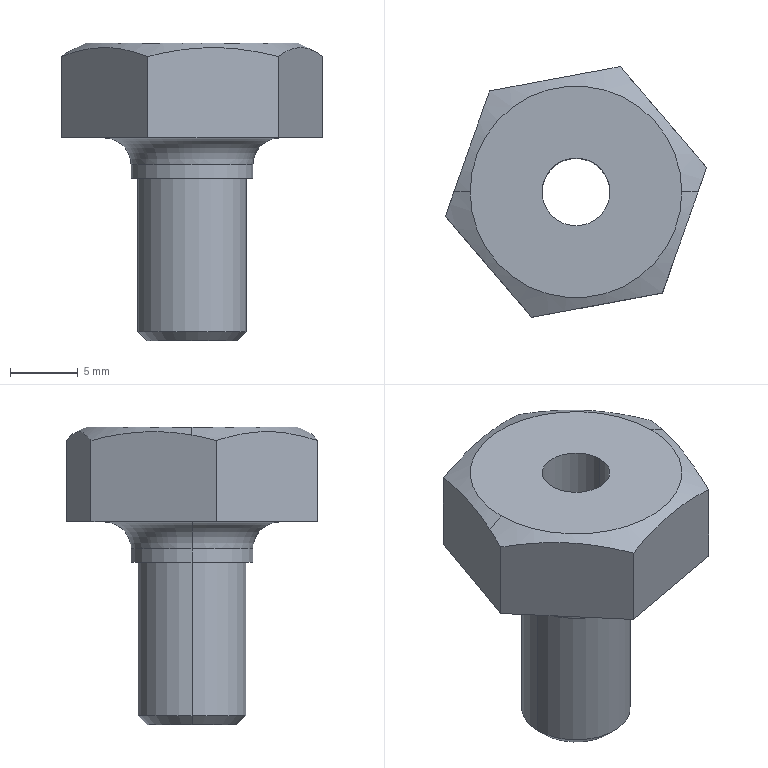Part | SolidWorks | features Cut 1, Extrusion 1, Fillet 1, ICE 1, RevCut 1, StudWizard 1 | 1 solid | 22 faces | box 19.298 x 18.51 x 22 mm | volume 2117 mm3 | plane 10 | cylinder 6 | cone 4 | torus 2 | commonest cylinder face diameters 5 x2 8 x2 9 x2
STEP:
#1=CARTESIAN_POINT('',(-124.031,115.619,-15.));
#2=VERTEX_POINT('',#1);
#3=CARTESIAN_POINT('',(-119.031,115.619,-15.));
#4=VERTEX_POINT('',#3);
#5=CARTESIAN_POINT('',(-121.531,115.619,-15.));
#6=DIRECTION('',(0.,0.,1.));
#7=DIRECTION('',(-1.,0.,0.));
#8=AXIS2_PLACEMENT_3D('',#5,#6,#7);
#9=CIRCLE('',#8,2.5);
#10=EDGE_CURVE('',#2,#4,#9,.T.);
#11=ORIENTED_EDGE('',*,*,#10,.F.);
#12=CARTESIAN_POINT('',(-124.031,115.619,7.));
#13=VERTEX_POINT('',#12);
#14=CARTESIAN_POINT('',(-124.031,115.619,-22.071));
#15=DIRECTION('',(0.,0.,1.));
#16=VECTOR('',#15,1000.);
#17=LINE('',#14,#16);
#18=EDGE_CURVE('',#2,#13,#17,.T.);
#19=ORIENTED_EDGE('',*,*,#18,.T.);
#20=CARTESIAN_POINT('',(-119.031,115.619,7.));
#21=VERTEX_POINT('',#20);
#22=CARTESIAN_POINT('',(-121.531,115.619,7.));
#23=DIRECTION('',(0.,0.,1.));
#24=DIRECTION('',(1.,0.,0.));
#25=AXIS2_PLACEMENT_3D('',#22,#23,#24);
#26=CIRCLE('',#25,2.5);
#27=EDGE_CURVE('',#13,#21,#26,.T.);
#28=ORIENTED_EDGE('',*,*,#27,.T.);
#29=CARTESIAN_POINT('',(-119.031,115.619,-22.071));
#30=DIRECTION('',(0.,0.,1.));
#31=VECTOR('',#30,1000.);
#32=LINE('',#29,#31);
#33=EDGE_CURVE('',#4,#21,#32,.T.);
#34=ORIENTED_EDGE('',*,*,#33,.F.);
#35=EDGE_LOOP('',(#11,#19,#28,#34));
#36=FACE_OUTER_BOUND('',#35,.T.);
#37=CARTESIAN_POINT('',(-121.531,115.619,-22.071));
#38=DIRECTION('',(0.,0.,1.));
#39=DIRECTION('',(1.,0.,0.));
#40=AXIS2_PLACEMENT_3D('',#37,#38,#39);
#41=CYLINDRICAL_SURFACE('',#40,2.5);
#42=ADVANCED_FACE('',(#36),#41,.F.);
#43=CARTESIAN_POINT('',(-118.208,115.619,-15.));
#44=VERTEX_POINT('',#43);
#45=CARTESIAN_POINT('',(-124.855,115.619,-15.));
#46=VERTEX_POINT('',#45);
#47=CARTESIAN_POINT('',(-121.531,115.619,-15.));
#48=DIRECTION('',(0.,0.,1.));
#49=DIRECTION('',(1.,0.,0.));
#50=AXIS2_PLACEMENT_3D('',#47,#48,#49);
#51=CIRCLE('',#50,3.324);
#52=EDGE_CURVE('',#44,#46,#51,.T.);
#53=ORIENTED_EDGE('',*,*,#52,.T.);
#54=CARTESIAN_POINT('',(-125.531,115.619,-14.324));
#55=VERTEX_POINT('',#54);
#56=CARTESIAN_POINT('',(-124.855,115.619,-15.));
#57=DIRECTION('',(-0.7071,0.,0.7071));
#58=VECTOR('',#57,1000.);
#59=LINE('',#56,#58);
#60=EDGE_CURVE('',#46,#55,#59,.T.);
#61=ORIENTED_EDGE('',*,*,#60,.T.);
#62=CARTESIAN_POINT('',(-117.531,115.619,-14.324));
#63=VERTEX_POINT('',#62);
#64=CARTESIAN_POINT('',(-121.531,115.619,-14.324));
#65=DIRECTION('',(0.,0.,1.));
#66=DIRECTION('',(1.,0.,0.));
#67=AXIS2_PLACEMENT_3D('',#64,#65,#66);
#68=CIRCLE('',#67,4.);
#69=EDGE_CURVE('',#63,#55,#68,.T.);
#70=ORIENTED_EDGE('',*,*,#69,.F.);
#71=CARTESIAN_POINT('',(-118.208,115.619,-15.));
#72=DIRECTION('',(0.7071,0.,0.7071));
#73=VECTOR('',#72,1000.);
#74=LINE('',#71,#73);
#75=EDGE_CURVE('',#44,#63,#74,.T.);
#76=ORIENTED_EDGE('',*,*,#75,.F.);
#77=EDGE_LOOP('',(#53,#61,#70,#76));
#78=FACE_OUTER_BOUND('',#77,.T.);
#79=CARTESIAN_POINT('',(-121.531,115.619,-15.));
#80=DIRECTION('',(0.,0.,1.));
#81=DIRECTION('',(1.,0.,0.));
#82=AXIS2_PLACEMENT_3D('',#79,#80,#81);
#83=CONICAL_SURFACE('',#82,3.324,0.7854);
#84=ADVANCED_FACE('',(#78),#83,.T.);
#85=ORIENTED_EDGE('',*,*,#69,.T.);
#86=CARTESIAN_POINT('',(-125.531,115.619,-3.));
#87=VERTEX_POINT('',#86);
#88=CARTESIAN_POINT('',(-125.531,115.619,-15.));
#89=DIRECTION('',(0.,0.,1.));
#90=VECTOR('',#89,1000.);
#91=LINE('',#88,#90);
#92=EDGE_CURVE('',#55,#87,#91,.T.);
#93=ORIENTED_EDGE('',*,*,#92,.T.);
#94=CARTESIAN_POINT('',(-117.531,115.619,-3.));
#95=VERTEX_POINT('',#94);
#96=CARTESIAN_POINT('',(-121.531,115.619,-3.));
#97=DIRECTION('',(0.,0.,1.));
#98=DIRECTION('',(1.,0.,0.));
#99=AXIS2_PLACEMENT_3D('',#96,#97,#98);
#100=CIRCLE('',#99,4.);
#101=EDGE_CURVE('',#95,#87,#100,.T.);
#102=ORIENTED_EDGE('',*,*,#101,.F.);
#103=CARTESIAN_POINT('',(-117.531,115.619,-15.));
#104=DIRECTION('',(0.,0.,1.));
#105=VECTOR('',#104,1000.);
#106=LINE('',#103,#105);
#107=EDGE_CURVE('',#63,#95,#106,.T.);
#108=ORIENTED_EDGE('',*,*,#107,.F.);
#109=EDGE_LOOP('',(#85,#93,#102,#108));
#110=FACE_OUTER_BOUND('',#109,.T.);
#111=CARTESIAN_POINT('',(-121.531,115.619,-15.));
#112=DIRECTION('',(0.,0.,1.));
#113=DIRECTION('',(1.,0.,0.));
#114=AXIS2_PLACEMENT_3D('',#111,#112,#113);
#115=CYLINDRICAL_SURFACE('',#114,4.);
#116=ADVANCED_FACE('',(#110),#115,.T.);
#117=CARTESIAN_POINT('',(-113.716,115.619,7.));
#118=VERTEX_POINT('',#117);
#119=CARTESIAN_POINT('',(-129.346,115.619,7.));
#120=VERTEX_POINT('',#119);
#121=CARTESIAN_POINT('',(-121.531,115.619,7.));
#122=DIRECTION('',(0.,0.,1.));
#123=DIRECTION('',(1.,0.,0.));
#124=AXIS2_PLACEMENT_3D('',#121,#122,#123);
#125=CIRCLE('',#124,7.815);
#126=EDGE_CURVE('',#118,#120,#125,.T.);
#127=ORIENTED_EDGE('',*,*,#126,.F.);
#128=CARTESIAN_POINT('',(-112.517,115.619,6.4));
#129=VERTEX_POINT('',#128);
#130=CARTESIAN_POINT('',(-113.716,115.619,7.));
#131=DIRECTION('',(0.8944,0.,-0.4472));
#132=VECTOR('',#131,1000.);
#133=LINE('',#130,#132);
#134=EDGE_CURVE('',#118,#129,#133,.T.);
#135=ORIENTED_EDGE('',*,*,#134,.T.);
#136=CARTESIAN_POINT('',(-111.882,117.417,6.));
#137=VERTEX_POINT('',#136);
#138=CARTESIAN_POINT('',(-112.517,115.619,6.4));
#139=CARTESIAN_POINT('',(-112.304,116.223,6.294));
#140=CARTESIAN_POINT('',(-112.092,116.822,6.158));
#141=CARTESIAN_POINT('',(-111.882,117.417,6.));
#142=B_SPLINE_CURVE_WITH_KNOTS('',3,(#138,#139,#140,#141),.UNSPECIFIED.,.F.,.F.,(4,4),(0.007924,0.009843),.UNSPECIFIED.);
#143=EDGE_CURVE('',#129,#137,#142,.T.);
#144=ORIENTED_EDGE('',*,*,#143,.T.);
#145=CARTESIAN_POINT('',(-118.263,124.874,6.));
#146=VERTEX_POINT('',#145);
#147=CARTESIAN_POINT('',(-111.882,117.417,6.));
#148=CARTESIAN_POINT('',(-112.406,118.029,6.202));
#149=CARTESIAN_POINT('',(-112.933,118.644,6.367));
#150=CARTESIAN_POINT('',(-113.99,119.88,6.594));
#151=CARTESIAN_POINT('',(-114.522,120.502,6.656));
#152=CARTESIAN_POINT('',(-115.325,121.44,6.658));
#153=CARTESIAN_POINT('',(-115.593,121.754,6.644));
#154=CARTESIAN_POINT('',(-116.132,122.383,6.585));
#155=CARTESIAN_POINT('',(-116.402,122.699,6.541));
#156=CARTESIAN_POINT('',(-117.207,123.639,6.369));
#157=CARTESIAN_POINT('',(-117.737,124.259,6.202));
#158=CARTESIAN_POINT('',(-118.263,124.874,6.));
#159=B_SPLINE_CURVE_WITH_KNOTS('',3,(#147,#148,#149,#150,#151,#152,#153,#154,#155,#156,#157,#158),.UNSPECIFIED.,.F.,.F.,(4,2,2,2,2,4),(0.000000268,0.002461,0.004922,0.006152,0.007382,0.009843),.UNSPECIFIED.);
#160=EDGE_CURVE('',#137,#146,#159,.T.);
#161=ORIENTED_EDGE('',*,*,#160,.T.);
#162=CARTESIAN_POINT('',(-127.912,123.076,6.));
#163=VERTEX_POINT('',#162);
#164=CARTESIAN_POINT('',(-118.263,124.874,6.));
#165=CARTESIAN_POINT('',(-119.056,124.726,6.202));
#166=CARTESIAN_POINT('',(-119.852,124.578,6.367));
#167=CARTESIAN_POINT('',(-121.451,124.28,6.594));
#168=CARTESIAN_POINT('',(-122.255,124.13,6.656));
#169=CARTESIAN_POINT('',(-123.469,123.904,6.658));
#170=CARTESIAN_POINT('',(-123.875,123.829,6.644));
#171=CARTESIAN_POINT('',(-124.689,123.677,6.585));
#172=CARTESIAN_POINT('',(-125.098,123.601,6.541));
#173=CARTESIAN_POINT('',(-126.315,123.374,6.369));
#174=CARTESIAN_POINT('',(-127.117,123.225,6.202));
#175=CARTESIAN_POINT('',(-127.912,123.076,6.));
#176=B_SPLINE_CURVE_WITH_KNOTS('',3,(#164,#165,#166,#167,#168,#169,#170,#171,#172,#173,#174,#175),.UNSPECIFIED.,.F.,.F.,(4,2,2,2,2,4),(0.000000207,0.002461,0.004922,0.006152,0.007382,0.009843),.UNSPECIFIED.);
#177=EDGE_CURVE('',#146,#163,#176,.T.);
#178=ORIENTED_EDGE('',*,*,#177,.T.);
#179=CARTESIAN_POINT('',(-130.545,115.619,6.4));
#180=VERTEX_POINT('',#179);
#181=CARTESIAN_POINT('',(-127.912,123.076,6.));
#182=CARTESIAN_POINT('',(-128.345,121.852,6.325));
#183=CARTESIAN_POINT('',(-128.779,120.621,6.553));
#184=CARTESIAN_POINT('',(-129.438,118.755,6.667));
#185=CARTESIAN_POINT('',(-129.659,118.13,6.667));
#186=CARTESIAN_POINT('',(-130.102,116.874,6.589));
#187=CARTESIAN_POINT('',(-130.325,116.242,6.51));
#188=CARTESIAN_POINT('',(-130.545,115.619,6.4));
#189=B_SPLINE_CURVE_WITH_KNOTS('',3,(#181,#182,#183,#184,#185,#186,#187,#188),.UNSPECIFIED.,.F.,.F.,(4,2,2,4),(0.000000216,0.003962,0.005943,0.007924),.UNSPECIFIED.);
#190=EDGE_CURVE('',#163,#180,#189,.T.);
#191=ORIENTED_EDGE('',*,*,#190,.T.);
#192=CARTESIAN_POINT('',(-129.346,115.619,7.));
#193=DIRECTION('',(-0.8944,0.,-0.4472));
#194=VECTOR('',#193,1000.);
#195=LINE('',#192,#194);
#196=EDGE_CURVE('',#120,#180,#195,.T.);
#197=ORIENTED_EDGE('',*,*,#196,.F.);
#198=EDGE_LOOP('',(#127,#135,#144,#161,#178,#191,#197));
#199=FACE_OUTER_BOUND('',#198,.T.);
#200=CARTESIAN_POINT('',(-121.531,115.619,7.));
#201=DIRECTION('',(0.,0.,-1.));
#202=DIRECTION('',(-1.,0.,0.));
#203=AXIS2_PLACEMENT_3D('',#200,#201,#202);
#204=CONICAL_SURFACE('',#203,7.815,1.107);
#205=ADVANCED_FACE('',(#199),#204,.T.);
#206=CARTESIAN_POINT('',(-128.031,115.619,0.));
#207=VERTEX_POINT('',#206);
#208=CARTESIAN_POINT('',(-115.031,115.619,0.));
#209=VERTEX_POINT('',#208);
#210=CARTESIAN_POINT('',(-121.531,115.619,0.));
#211=DIRECTION('',(0.,0.,1.));
#212=DIRECTION('',(1.,0.,0.));
#213=AXIS2_PLACEMENT_3D('',#210,#211,#212);
#214=CIRCLE('',#213,6.5);
#215=EDGE_CURVE('',#207,#209,#214,.T.);
#216=ORIENTED_EDGE('',*,*,#215,.F.);
#217=CARTESIAN_POINT('',(-126.031,115.619,-2.));
#218=VERTEX_POINT('',#217);
#219=CARTESIAN_POINT('',(-128.031,115.619,-2.));
#220=DIRECTION('',(0.,1.,0.));
#221=DIRECTION('',(-1.,0.,0.));
#222=AXIS2_PLACEMENT_3D('',#219,#220,#221);
#223=CIRCLE('',#222,2.);
#224=EDGE_CURVE('',#207,#218,#223,.T.);
#225=ORIENTED_EDGE('',*,*,#224,.T.);
#226=CARTESIAN_POINT('',(-117.031,115.619,-2.));
#227=VERTEX_POINT('',#226);
#228=CARTESIAN_POINT('',(-121.531,115.619,-2.));
#229=DIRECTION('',(0.,0.,-1.));
#230=DIRECTION('',(1.,0.,0.));
#231=AXIS2_PLACEMENT_3D('',#228,#229,#230);
#232=CIRCLE('',#231,4.5);
#233=EDGE_CURVE('',#227,#218,#232,.T.);
#234=ORIENTED_EDGE('',*,*,#233,.F.);
#235=CARTESIAN_POINT('',(-115.031,115.619,-2.));
#236=DIRECTION('',(0.,-1.,0.));
#237=DIRECTION('',(0.,0.,-1.));
#238=AXIS2_PLACEMENT_3D('',#235,#236,#237);
#239=CIRCLE('',#238,2.);
#240=EDGE_CURVE('',#209,#227,#239,.T.);
#241=ORIENTED_EDGE('',*,*,#240,.F.);
#242=EDGE_LOOP('',(#216,#225,#234,#241));
#243=FACE_OUTER_BOUND('',#242,.T.);
#244=CARTESIAN_POINT('',(-121.531,115.619,-2.));
#245=DIRECTION('',(0.,0.,1.));
#246=DIRECTION('',(1.,0.,0.));
#247=AXIS2_PLACEMENT_3D('',#244,#245,#246);
#248=TOROIDAL_SURFACE('',#247,6.5,2.);
#249=ADVANCED_FACE('',(#243),#248,.F.);
#250=CARTESIAN_POINT('',(-117.031,115.619,-3.));
#251=VERTEX_POINT('',#250);
#252=CARTESIAN_POINT('',(-126.031,115.619,-3.));
#253=VERTEX_POINT('',#252);
#254=CARTESIAN_POINT('',(-121.531,115.619,-3.));
#255=DIRECTION('',(0.,0.,1.));
#256=DIRECTION('',(1.,0.,0.));
#257=AXIS2_PLACEMENT_3D('',#254,#255,#256);
#258=CIRCLE('',#257,4.5);
#259=EDGE_CURVE('',#251,#253,#258,.T.);
#260=ORIENTED_EDGE('',*,*,#259,.T.);
#261=CARTESIAN_POINT('',(-126.031,115.619,-15.));
#262=DIRECTION('',(0.,0.,1.));
#263=VECTOR('',#262,1000.);
#264=LINE('',#261,#263);
#265=EDGE_CURVE('',#253,#218,#264,.T.);
#266=ORIENTED_EDGE('',*,*,#265,.T.);
#267=CARTESIAN_POINT('',(-121.531,115.619,-2.));
#268=DIRECTION('',(0.,0.,-1.));
#269=DIRECTION('',(1.,0.,0.));
#270=AXIS2_PLACEMENT_3D('',#267,#268,#269);
#271=CIRCLE('',#270,4.5);
#272=EDGE_CURVE('',#218,#227,#271,.T.);
#273=ORIENTED_EDGE('',*,*,#272,.T.);
#274=CARTESIAN_POINT('',(-117.031,115.619,-15.));
#275=DIRECTION('',(0.,0.,1.));
#276=VECTOR('',#275,1000.);
#277=LINE('',#274,#276);
#278=EDGE_CURVE('',#251,#227,#277,.T.);
#279=ORIENTED_EDGE('',*,*,#278,.F.);
#280=EDGE_LOOP('',(#260,#266,#273,#279));
#281=FACE_OUTER_BOUND('',#280,.T.);
#282=CARTESIAN_POINT('',(-121.531,115.619,-15.));
#283=DIRECTION('',(0.,0.,1.));
#284=DIRECTION('',(1.,0.,0.));
#285=AXIS2_PLACEMENT_3D('',#282,#283,#284);
#286=CYLINDRICAL_SURFACE('',#285,4.5);
#287=ADVANCED_FACE('',(#281),#286,.T.);
#288=CARTESIAN_POINT('',(-124.799,106.364,6.));
#289=VERTEX_POINT('',#288);
#290=CARTESIAN_POINT('',(-115.15,108.162,6.));
#291=VERTEX_POINT('',#290);
#292=CARTESIAN_POINT('',(-124.799,106.364,6.));
#293=CARTESIAN_POINT('',(-124.006,106.512,6.202));
#294=CARTESIAN_POINT('',(-123.211,106.66,6.367));
#295=CARTESIAN_POINT('',(-121.611,106.958,6.594));
#296=CARTESIAN_POINT('',(-120.807,107.108,6.656));
#297=CARTESIAN_POINT('',(-119.593,107.334,6.658));
#298=CARTESIAN_POINT('',(-119.187,107.409,6.644));
#299=CARTESIAN_POINT('',(-118.373,107.561,6.585));
#300=CARTESIAN_POINT('',(-117.964,107.637,6.541));
#301=CARTESIAN_POINT('',(-116.748,107.864,6.369));
#302=CARTESIAN_POINT('',(-115.946,108.013,6.202));
#303=CARTESIAN_POINT('',(-115.15,108.162,6.));
#304=B_SPLINE_CURVE_WITH_KNOTS('',3,(#292,#293,#294,#295,#296,#297,#298,#299,#300,#301,#302,#303),.UNSPECIFIED.,.F.,.F.,(4,2,2,2,2,4),(0.000000207,0.002461,0.004922,0.006152,0.007382,0.009843),.UNSPECIFIED.);
#305=EDGE_CURVE('',#289,#291,#304,.T.);
#306=ORIENTED_EDGE('',*,*,#305,.F.);
#307=CARTESIAN_POINT('',(-124.799,106.364,0.));
#308=VERTEX_POINT('',#307);
#309=CARTESIAN_POINT('',(-124.799,106.364,7.));
#310=DIRECTION('',(0.,0.,-1.));
#311=VECTOR('',#310,1000.);
#312=LINE('',#309,#311);
#313=EDGE_CURVE('',#289,#308,#312,.T.);
#314=ORIENTED_EDGE('',*,*,#313,.T.);
#315=CARTESIAN_POINT('',(-115.15,108.162,0.));
#316=VERTEX_POINT('',#315);
#317=CARTESIAN_POINT('',(-119.974,107.263,0.));
#318=DIRECTION('',(0.9831,0.1831,0.));
#319=VECTOR('',#318,1000.);
#320=LINE('',#317,#319);
#321=EDGE_CURVE('',#308,#316,#320,.T.);
#322=ORIENTED_EDGE('',*,*,#321,.T.);
#323=CARTESIAN_POINT('',(-115.15,108.162,7.));
#324=DIRECTION('',(0.,0.,-1.));
#325=VECTOR('',#324,1000.);
#326=LINE('',#323,#325);
#327=EDGE_CURVE('',#291,#316,#326,.T.);
#328=ORIENTED_EDGE('',*,*,#327,.F.);
#329=EDGE_LOOP('',(#306,#314,#322,#328));
#330=FACE_OUTER_BOUND('',#329,.T.);
#331=CARTESIAN_POINT('',(-119.974,107.263,7.));
#332=DIRECTION('',(-0.1831,0.9831,0.));
#333=DIRECTION('',(-0.9831,-0.1831,0.));
#334=AXIS2_PLACEMENT_3D('',#331,#332,#333);
#335=PLANE('',#334);
#336=ADVANCED_FACE('',(#330),#335,.F.);
#337=CARTESIAN_POINT('',(-115.15,108.162,6.));
#338=CARTESIAN_POINT('',(-114.718,109.386,6.325));
#339=CARTESIAN_POINT('',(-114.283,110.617,6.553));
#340=CARTESIAN_POINT('',(-113.624,112.483,6.667));
#341=CARTESIAN_POINT('',(-113.404,113.108,6.667));
#342=CARTESIAN_POINT('',(-112.96,114.364,6.589));
#343=CARTESIAN_POINT('',(-112.737,114.996,6.51));
#344=CARTESIAN_POINT('',(-112.517,115.619,6.4));
#345=B_SPLINE_CURVE_WITH_KNOTS('',3,(#337,#338,#339,#340,#341,#342,#343,#344),.UNSPECIFIED.,.F.,.F.,(4,2,2,4),(0.000000216,0.003962,0.005943,0.007924),.UNSPECIFIED.);
#346=EDGE_CURVE('',#291,#129,#345,.T.);
#347=ORIENTED_EDGE('',*,*,#346,.F.);
#348=ORIENTED_EDGE('',*,*,#327,.T.);
#349=CARTESIAN_POINT('',(-111.882,117.417,0.));
#350=VERTEX_POINT('',#349);
#351=CARTESIAN_POINT('',(-113.516,112.789,0.));
#352=DIRECTION('',(0.3329,0.943,0.));
#353=VECTOR('',#352,1000.);
#354=LINE('',#351,#353);
#355=EDGE_CURVE('',#316,#350,#354,.T.);
#356=ORIENTED_EDGE('',*,*,#355,.T.);
#357=CARTESIAN_POINT('',(-111.882,117.417,7.));
#358=DIRECTION('',(0.,0.,-1.));
#359=VECTOR('',#358,1000.);
#360=LINE('',#357,#359);
#361=EDGE_CURVE('',#137,#350,#360,.T.);
#362=ORIENTED_EDGE('',*,*,#361,.F.);
#363=ORIENTED_EDGE('',*,*,#143,.F.);
#364=EDGE_LOOP('',(#347,#348,#356,#362,#363));
#365=FACE_OUTER_BOUND('',#364,.T.);
#366=CARTESIAN_POINT('',(-113.516,112.789,7.));
#367=DIRECTION('',(-0.943,0.3329,0.));
#368=DIRECTION('',(-0.3329,-0.943,0.));
#369=AXIS2_PLACEMENT_3D('',#366,#367,#368);
#370=PLANE('',#369);
#371=ADVANCED_FACE('',(#365),#370,.F.);
#372=ORIENTED_EDGE('',*,*,#160,.F.);
#373=ORIENTED_EDGE('',*,*,#361,.T.);
#374=CARTESIAN_POINT('',(-118.263,124.874,0.));
#375=VERTEX_POINT('',#374);
#376=CARTESIAN_POINT('',(-115.073,121.145,0.));
#377=DIRECTION('',(-0.6502,0.7598,0.));
#378=VECTOR('',#377,1000.);
#379=LINE('',#376,#378);
#380=EDGE_CURVE('',#350,#375,#379,.T.);
#381=ORIENTED_EDGE('',*,*,#380,.T.);
#382=CARTESIAN_POINT('',(-118.263,124.874,7.));
#383=DIRECTION('',(0.,0.,-1.));
#384=VECTOR('',#383,1000.);
#385=LINE('',#382,#384);
#386=EDGE_CURVE('',#146,#375,#385,.T.);
#387=ORIENTED_EDGE('',*,*,#386,.F.);
#388=EDGE_LOOP('',(#372,#373,#381,#387));
#389=FACE_OUTER_BOUND('',#388,.T.);
#390=CARTESIAN_POINT('',(-115.073,121.145,7.));
#391=DIRECTION('',(-0.7598,-0.6502,0.));
#392=DIRECTION('',(0.6502,-0.7598,0.));
#393=AXIS2_PLACEMENT_3D('',#390,#391,#392);
#394=PLANE('',#393);
#395=ADVANCED_FACE('',(#389),#394,.F.);
#396=ORIENTED_EDGE('',*,*,#177,.F.);
#397=ORIENTED_EDGE('',*,*,#386,.T.);
#398=CARTESIAN_POINT('',(-127.912,123.076,0.));
#399=VERTEX_POINT('',#398);
#400=CARTESIAN_POINT('',(-123.088,123.975,0.));
#401=DIRECTION('',(-0.9831,-0.1831,0.));
#402=VECTOR('',#401,1000.);
#403=LINE('',#400,#402);
#404=EDGE_CURVE('',#375,#399,#403,.T.);
#405=ORIENTED_EDGE('',*,*,#404,.T.);
#406=CARTESIAN_POINT('',(-127.912,123.076,7.));
#407=DIRECTION('',(0.,0.,-1.));
#408=VECTOR('',#407,1000.);
#409=LINE('',#406,#408);
#410=EDGE_CURVE('',#163,#399,#409,.T.);
#411=ORIENTED_EDGE('',*,*,#410,.F.);
#412=EDGE_LOOP('',(#396,#397,#405,#411));
#413=FACE_OUTER_BOUND('',#412,.T.);
#414=CARTESIAN_POINT('',(-123.088,123.975,7.));
#415=DIRECTION('',(0.1831,-0.9831,0.));
#416=DIRECTION('',(0.9831,0.1831,0.));
#417=AXIS2_PLACEMENT_3D('',#414,#415,#416);
#418=PLANE('',#417);
#419=ADVANCED_FACE('',(#413),#418,.F.);
#420=ORIENTED_EDGE('',*,*,#190,.F.);
#421=ORIENTED_EDGE('',*,*,#410,.T.);
#422=CARTESIAN_POINT('',(-131.18,113.821,0.));
#423=VERTEX_POINT('',#422);
#424=CARTESIAN_POINT('',(-129.546,118.449,0.));
#425=DIRECTION('',(-0.3329,-0.943,0.));
#426=VECTOR('',#425,1000.);
#427=LINE('',#424,#426);
#428=EDGE_CURVE('',#399,#423,#427,.T.);
#429=ORIENTED_EDGE('',*,*,#428,.T.);
#430=CARTESIAN_POINT('',(-131.18,113.821,6.));
#431=VERTEX_POINT('',#430);
#432=CARTESIAN_POINT('',(-131.18,113.821,7.));
#433=DIRECTION('',(0.,0.,-1.));
#434=VECTOR('',#433,1000.);
#435=LINE('',#432,#434);
#436=EDGE_CURVE('',#431,#423,#435,.T.);
#437=ORIENTED_EDGE('',*,*,#436,.F.);
#438=CARTESIAN_POINT('',(-130.545,115.619,6.4));
#439=CARTESIAN_POINT('',(-130.759,115.015,6.294));
#440=CARTESIAN_POINT('',(-130.97,114.416,6.158));
#441=CARTESIAN_POINT('',(-131.18,113.821,6.));
#442=B_SPLINE_CURVE_WITH_KNOTS('',3,(#438,#439,#440,#441),.UNSPECIFIED.,.F.,.F.,(4,4),(0.007924,0.009843),.UNSPECIFIED.);
#443=EDGE_CURVE('',#180,#431,#442,.T.);
#444=ORIENTED_EDGE('',*,*,#443,.F.);
#445=EDGE_LOOP('',(#420,#421,#429,#437,#444));
#446=FACE_OUTER_BOUND('',#445,.T.);
#447=CARTESIAN_POINT('',(-129.546,118.449,7.));
#448=DIRECTION('',(0.943,-0.3329,0.));
#449=DIRECTION('',(0.3329,0.943,0.));
#450=AXIS2_PLACEMENT_3D('',#447,#448,#449);
#451=PLANE('',#450);
#452=ADVANCED_FACE('',(#446),#451,.F.);
#453=CARTESIAN_POINT('',(-131.18,113.821,6.));
#454=CARTESIAN_POINT('',(-130.656,113.209,6.202));
#455=CARTESIAN_POINT('',(-130.13,112.594,6.367));
#456=CARTESIAN_POINT('',(-129.072,111.358,6.594));
#457=CARTESIAN_POINT('',(-128.54,110.736,6.656));
#458=CARTESIAN_POINT('',(-127.737,109.798,6.658));
#459=CARTESIAN_POINT('',(-127.469,109.485,6.644));
#460=CARTESIAN_POINT('',(-126.931,108.855,6.585));
#461=CARTESIAN_POINT('',(-126.66,108.539,6.541));
#462=CARTESIAN_POINT('',(-125.855,107.599,6.369));
#463=CARTESIAN_POINT('',(-125.325,106.979,6.202));
#464=CARTESIAN_POINT('',(-124.799,106.364,6.));
#465=B_SPLINE_CURVE_WITH_KNOTS('',3,(#453,#454,#455,#456,#457,#458,#459,#460,#461,#462,#463,#464),.UNSPECIFIED.,.F.,.F.,(4,2,2,2,2,4),(0.000000268,0.002461,0.004922,0.006152,0.007382,0.009843),.UNSPECIFIED.);
#466=EDGE_CURVE('',#431,#289,#465,.T.);
#467=ORIENTED_EDGE('',*,*,#466,.F.);
#468=ORIENTED_EDGE('',*,*,#436,.T.);
#469=CARTESIAN_POINT('',(-127.989,110.093,0.));
#470=DIRECTION('',(0.6502,-0.7598,0.));
#471=VECTOR('',#470,1000.);
#472=LINE('',#469,#471);
#473=EDGE_CURVE('',#423,#308,#472,.T.);
#474=ORIENTED_EDGE('',*,*,#473,.T.);
#475=ORIENTED_EDGE('',*,*,#313,.F.);
#476=EDGE_LOOP('',(#467,#468,#474,#475));
#477=FACE_OUTER_BOUND('',#476,.T.);
#478=CARTESIAN_POINT('',(-127.989,110.093,7.));
#479=DIRECTION('',(0.7598,0.6502,0.));
#480=DIRECTION('',(-0.6502,0.7598,0.));
#481=AXIS2_PLACEMENT_3D('',#478,#479,#480);
#482=PLANE('',#481);
#483=ADVANCED_FACE('',(#477),#482,.F.);
#484=CARTESIAN_POINT('',(-121.531,115.619,0.));
#485=DIRECTION('',(0.,0.,1.));
#486=DIRECTION('',(1.,0.,0.));
#487=AXIS2_PLACEMENT_3D('',#484,#485,#486);
#488=CIRCLE('',#487,6.5);
#489=EDGE_CURVE('',#209,#207,#488,.T.);
#490=ORIENTED_EDGE('',*,*,#489,.T.);
#491=ORIENTED_EDGE('',*,*,#215,.T.);
#492=EDGE_LOOP('',(#490,#491));
#493=FACE_BOUND('',#492,.T.);
#494=ORIENTED_EDGE('',*,*,#321,.F.);
#495=ORIENTED_EDGE('',*,*,#473,.F.);
#496=ORIENTED_EDGE('',*,*,#428,.F.);
#497=ORIENTED_EDGE('',*,*,#404,.F.);
#498=ORIENTED_EDGE('',*,*,#380,.F.);
#499=ORIENTED_EDGE('',*,*,#355,.F.);
#500=EDGE_LOOP('',(#494,#495,#496,#497,#498,#499));
#501=FACE_OUTER_BOUND('',#500,.T.);
#502=CARTESIAN_POINT('',(0.,0.,0.));
#503=DIRECTION('',(0.,0.,1.));
#504=DIRECTION('',(1.,0.,0.));
#505=AXIS2_PLACEMENT_3D('',#502,#503,#504);
#506=PLANE('',#505);
#507=ADVANCED_FACE('',(#493,#501),#506,.F.);
#508=ORIENTED_EDGE('',*,*,#265,.F.);
#509=CARTESIAN_POINT('',(-121.531,115.619,-3.));
#510=DIRECTION('',(0.,0.,1.));
#511=DIRECTION('',(1.,0.,0.));
#512=AXIS2_PLACEMENT_3D('',#509,#510,#511);
#513=CIRCLE('',#512,4.5);
#514=EDGE_CURVE('',#253,#251,#513,.T.);
#515=ORIENTED_EDGE('',*,*,#514,.T.);
#516=ORIENTED_EDGE('',*,*,#278,.T.);
#517=ORIENTED_EDGE('',*,*,#233,.T.);
#518=EDGE_LOOP('',(#508,#515,#516,#517));
#519=FACE_OUTER_BOUND('',#518,.T.);
#520=CARTESIAN_POINT('',(-121.531,115.619,-15.));
#521=DIRECTION('',(0.,0.,1.));
#522=DIRECTION('',(1.,0.,0.));
#523=AXIS2_PLACEMENT_3D('',#520,#521,#522);
#524=CYLINDRICAL_SURFACE('',#523,4.5);
#525=ADVANCED_FACE('',(#519),#524,.T.);
#526=ORIENTED_EDGE('',*,*,#224,.F.);
#527=ORIENTED_EDGE('',*,*,#489,.F.);
#528=ORIENTED_EDGE('',*,*,#240,.T.);
#529=ORIENTED_EDGE('',*,*,#272,.F.);
#530=EDGE_LOOP('',(#526,#527,#528,#529));
#531=FACE_OUTER_BOUND('',#530,.T.);
#532=CARTESIAN_POINT('',(-121.531,115.619,-2.));
#533=DIRECTION('',(0.,0.,1.));
#534=DIRECTION('',(1.,0.,0.));
#535=AXIS2_PLACEMENT_3D('',#532,#533,#534);
#536=TOROIDAL_SURFACE('',#535,6.5,2.);
#537=ADVANCED_FACE('',(#531),#536,.F.);
#538=ORIENTED_EDGE('',*,*,#134,.F.);
#539=CARTESIAN_POINT('',(-121.531,115.619,7.));
#540=DIRECTION('',(0.,0.,1.));
#541=DIRECTION('',(1.,0.,0.));
#542=AXIS2_PLACEMENT_3D('',#539,#540,#541);
#543=CIRCLE('',#542,7.815);
#544=EDGE_CURVE('',#120,#118,#543,.T.);
#545=ORIENTED_EDGE('',*,*,#544,.F.);
#546=ORIENTED_EDGE('',*,*,#196,.T.);
#547=ORIENTED_EDGE('',*,*,#443,.T.);
#548=ORIENTED_EDGE('',*,*,#466,.T.);
#549=ORIENTED_EDGE('',*,*,#305,.T.);
#550=ORIENTED_EDGE('',*,*,#346,.T.);
#551=EDGE_LOOP('',(#538,#545,#546,#547,#548,#549,#550));
#552=FACE_OUTER_BOUND('',#551,.T.);
#553=CARTESIAN_POINT('',(-121.531,115.619,7.));
#554=DIRECTION('',(0.,0.,-1.));
#555=DIRECTION('',(-1.,0.,0.));
#556=AXIS2_PLACEMENT_3D('',#553,#554,#555);
#557=CONICAL_SURFACE('',#556,7.815,1.107);
#558=ADVANCED_FACE('',(#552),#557,.T.);
#559=CARTESIAN_POINT('',(-121.531,115.619,7.));
#560=DIRECTION('',(0.,0.,1.));
#561=DIRECTION('',(1.,0.,0.));
#562=AXIS2_PLACEMENT_3D('',#559,#560,#561);
#563=CIRCLE('',#562,2.5);
#564=EDGE_CURVE('',#21,#13,#563,.T.);
#565=ORIENTED_EDGE('',*,*,#564,.F.);
#566=ORIENTED_EDGE('',*,*,#27,.F.);
#567=EDGE_LOOP('',(#565,#566));
#568=FACE_BOUND('',#567,.T.);
#569=ORIENTED_EDGE('',*,*,#544,.T.);
#570=ORIENTED_EDGE('',*,*,#126,.T.);
#571=EDGE_LOOP('',(#569,#570));
#572=FACE_OUTER_BOUND('',#571,.T.);
#573=CARTESIAN_POINT('',(0.,0.,7.));
#574=DIRECTION('',(0.,0.,1.));
#575=DIRECTION('',(1.,0.,0.));
#576=AXIS2_PLACEMENT_3D('',#573,#574,#575);
#577=PLANE('',#576);
#578=ADVANCED_FACE('',(#568,#572),#577,.T.);
#579=ORIENTED_EDGE('',*,*,#92,.F.);
#580=CARTESIAN_POINT('',(-121.531,115.619,-14.324));
#581=DIRECTION('',(0.,0.,1.));
#582=DIRECTION('',(1.,0.,0.));
#583=AXIS2_PLACEMENT_3D('',#580,#581,#582);
#584=CIRCLE('',#583,4.);
#585=EDGE_CURVE('',#55,#63,#584,.T.);
#586=ORIENTED_EDGE('',*,*,#585,.T.);
#587=ORIENTED_EDGE('',*,*,#107,.T.);
#588=CARTESIAN_POINT('',(-121.531,115.619,-3.));
#589=DIRECTION('',(0.,0.,1.));
#590=DIRECTION('',(1.,0.,0.));
#591=AXIS2_PLACEMENT_3D('',#588,#589,#590);
#592=CIRCLE('',#591,4.);
#593=EDGE_CURVE('',#87,#95,#592,.T.);
#594=ORIENTED_EDGE('',*,*,#593,.F.);
#595=EDGE_LOOP('',(#579,#586,#587,#594));
#596=FACE_OUTER_BOUND('',#595,.T.);
#597=CARTESIAN_POINT('',(-121.531,115.619,-15.));
#598=DIRECTION('',(0.,0.,1.));
#599=DIRECTION('',(1.,0.,0.));
#600=AXIS2_PLACEMENT_3D('',#597,#598,#599);
#601=CYLINDRICAL_SURFACE('',#600,4.);
#602=ADVANCED_FACE('',(#596),#601,.T.);
#603=ORIENTED_EDGE('',*,*,#259,.F.);
#604=ORIENTED_EDGE('',*,*,#514,.F.);
#605=EDGE_LOOP('',(#603,#604));
#606=FACE_OUTER_BOUND('',#605,.T.);
#607=ORIENTED_EDGE('',*,*,#101,.T.);
#608=ORIENTED_EDGE('',*,*,#593,.T.);
#609=EDGE_LOOP('',(#607,#608));
#610=FACE_BOUND('',#609,.T.);
#611=CARTESIAN_POINT('',(-117.531,115.619,-3.));
#612=DIRECTION('',(0.,0.,1.));
#613=DIRECTION('',(1.,0.,0.));
#614=AXIS2_PLACEMENT_3D('',#611,#612,#613);
#615=PLANE('',#614);
#616=ADVANCED_FACE('',(#606,#610),#615,.F.);
#617=ORIENTED_EDGE('',*,*,#60,.F.);
#618=CARTESIAN_POINT('',(-121.531,115.619,-15.));
#619=DIRECTION('',(0.,0.,1.));
#620=DIRECTION('',(1.,0.,0.));
#621=AXIS2_PLACEMENT_3D('',#618,#619,#620);
#622=CIRCLE('',#621,3.324);
#623=EDGE_CURVE('',#46,#44,#622,.T.);
#624=ORIENTED_EDGE('',*,*,#623,.T.);
#625=ORIENTED_EDGE('',*,*,#75,.T.);
#626=ORIENTED_EDGE('',*,*,#585,.F.);
#627=EDGE_LOOP('',(#617,#624,#625,#626));
#628=FACE_OUTER_BOUND('',#627,.T.);
#629=CARTESIAN_POINT('',(-121.531,115.619,-15.));
#630=DIRECTION('',(0.,0.,1.));
#631=DIRECTION('',(1.,0.,0.));
#632=AXIS2_PLACEMENT_3D('',#629,#630,#631);
#633=CONICAL_SURFACE('',#632,3.324,0.7854);
#634=ADVANCED_FACE('',(#628),#633,.T.);
#635=CARTESIAN_POINT('',(-121.531,115.619,-15.));
#636=DIRECTION('',(0.,0.,1.));
#637=DIRECTION('',(-1.,0.,0.));
#638=AXIS2_PLACEMENT_3D('',#635,#636,#637);
#639=CIRCLE('',#638,2.5);
#640=EDGE_CURVE('',#4,#2,#639,.T.);
#641=ORIENTED_EDGE('',*,*,#640,.T.);
#642=ORIENTED_EDGE('',*,*,#10,.T.);
#643=EDGE_LOOP('',(#641,#642));
#644=FACE_BOUND('',#643,.T.);
#645=ORIENTED_EDGE('',*,*,#52,.F.);
#646=ORIENTED_EDGE('',*,*,#623,.F.);
#647=EDGE_LOOP('',(#645,#646));
#648=FACE_OUTER_BOUND('',#647,.T.);
#649=CARTESIAN_POINT('',(-121.531,115.619,-15.));
#650=DIRECTION('',(0.,0.,-1.));
#651=DIRECTION('',(-1.,0.,0.));
#652=AXIS2_PLACEMENT_3D('',#649,#650,#651);
#653=PLANE('',#652);
#654=ADVANCED_FACE('',(#644,#648),#653,.T.);
#655=ORIENTED_EDGE('',*,*,#18,.F.);
#656=ORIENTED_EDGE('',*,*,#640,.F.);
#657=ORIENTED_EDGE('',*,*,#33,.T.);
#658=ORIENTED_EDGE('',*,*,#564,.T.);
#659=EDGE_LOOP('',(#655,#656,#657,#658));
#660=FACE_OUTER_BOUND('',#659,.T.);
#661=CARTESIAN_POINT('',(-121.531,115.619,-22.071));
#662=DIRECTION('',(0.,0.,1.));
#663=DIRECTION('',(1.,0.,0.));
#664=AXIS2_PLACEMENT_3D('',#661,#662,#663);
#665=CYLINDRICAL_SURFACE('',#664,2.5);
#666=ADVANCED_FACE('',(#660),#665,.F.);
#667=CLOSED_SHELL('',(#42,#84,#116,#205,#249,#287,#336,#371,#395,#419,#452,#483,#507,#525,#537,#558,#578,#602,#616,#634,#654,#666));
#668=MANIFOLD_SOLID_BREP('',#667);
#669=CARTESIAN_POINT('',(0.,0.,0.));
#670=DIRECTION('',(0.,0.,1.));
#671=DIRECTION('',(1.,0.,0.));
#672=AXIS2_PLACEMENT_3D('',#669,#670,#671);
#673=(LENGTH_UNIT()NAMED_UNIT(*)SI_UNIT(.MILLI.,.METRE.));
#674=UNCERTAINTY_MEASURE_WITH_UNIT(LENGTH_MEASURE(0.00001),#673,'','');
#675=(NAMED_UNIT(*)PLANE_ANGLE_UNIT()SI_UNIT($,.RADIAN.));
#676=(NAMED_UNIT(*)SI_UNIT($,.STERADIAN.)SOLID_ANGLE_UNIT());
#677=(GEOMETRIC_REPRESENTATION_CONTEXT(3)GLOBAL_UNCERTAINTY_ASSIGNED_CONTEXT((#674))GLOBAL_UNIT_ASSIGNED_CONTEXT((#673,#675,#676))REPRESENTATION_CONTEXT('',''));
#678=ADVANCED_BREP_SHAPE_REPRESENTATION('',(#668,#672),#677);